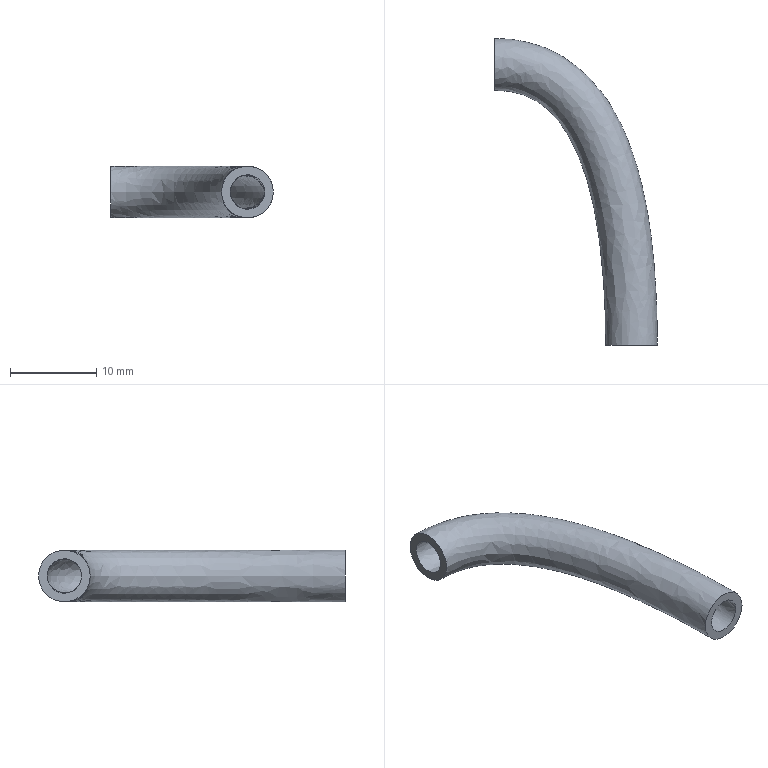Part | NX | features solid 2 | 1 solid | 4 faces | box 18.875 x 35.617 x 6 mm | volume 633.371 mm3 | plane 2 | spline 2